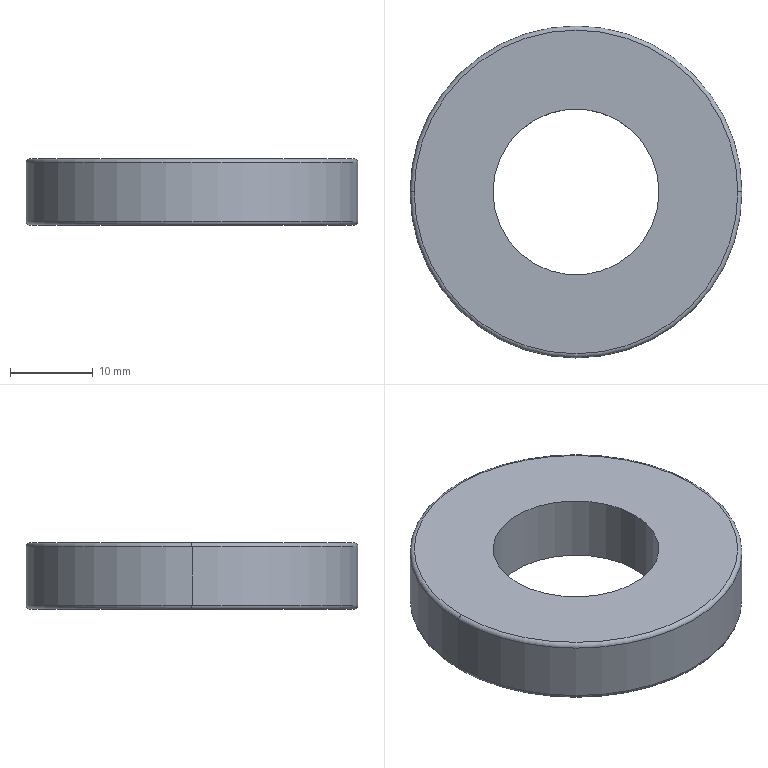Part | SolidWorks | features Extrusion 1, Fillet 1 | 1 solid | 10 faces | box 40 x 40 x 8 mm | volume 7526 mm3 | torus 4 | cylinder 4 | plane 2 | commonest cylinder face diameters 20 x2 40 x2
STEP:
#1=CARTESIAN_POINT('',(-20.,0.,3.5));
#2=VERTEX_POINT('',#1);
#3=CARTESIAN_POINT('',(20.,0.,3.5));
#4=VERTEX_POINT('',#3);
#5=CARTESIAN_POINT('',(0.,0.,3.5));
#6=DIRECTION('',(0.,0.,-1.));
#7=DIRECTION('',(1.,0.,0.));
#8=AXIS2_PLACEMENT_3D('',#5,#6,#7);
#9=CIRCLE('',#8,20.);
#10=EDGE_CURVE('',#2,#4,#9,.T.);
#11=ORIENTED_EDGE('',*,*,#10,.F.);
#12=CARTESIAN_POINT('',(-19.5,0.,4.));
#13=VERTEX_POINT('',#12);
#14=CARTESIAN_POINT('',(-19.5,0.,3.5));
#15=DIRECTION('',(0.,1.,0.));
#16=DIRECTION('',(-1.,0.,0.));
#17=AXIS2_PLACEMENT_3D('',#14,#15,#16);
#18=CIRCLE('',#17,0.5);
#19=EDGE_CURVE('',#2,#13,#18,.T.);
#20=ORIENTED_EDGE('',*,*,#19,.T.);
#21=CARTESIAN_POINT('',(19.5,0.,4.));
#22=VERTEX_POINT('',#21);
#23=CARTESIAN_POINT('',(0.,0.,4.));
#24=DIRECTION('',(0.,0.,1.));
#25=DIRECTION('',(1.,0.,0.));
#26=AXIS2_PLACEMENT_3D('',#23,#24,#25);
#27=CIRCLE('',#26,19.5);
#28=EDGE_CURVE('',#22,#13,#27,.T.);
#29=ORIENTED_EDGE('',*,*,#28,.F.);
#30=CARTESIAN_POINT('',(19.5,0.,3.5));
#31=DIRECTION('',(0.,-1.,0.));
#32=DIRECTION('',(0.,0.,-1.));
#33=AXIS2_PLACEMENT_3D('',#30,#31,#32);
#34=CIRCLE('',#33,0.5);
#35=EDGE_CURVE('',#4,#22,#34,.T.);
#36=ORIENTED_EDGE('',*,*,#35,.F.);
#37=EDGE_LOOP('',(#11,#20,#29,#36));
#38=FACE_OUTER_BOUND('',#37,.T.);
#39=CARTESIAN_POINT('',(0.,0.,3.5));
#40=DIRECTION('',(0.,0.,1.));
#41=DIRECTION('',(1.,0.,0.));
#42=AXIS2_PLACEMENT_3D('',#39,#40,#41);
#43=TOROIDAL_SURFACE('',#42,19.5,0.5);
#44=ADVANCED_FACE('',(#38),#43,.T.);
#45=CARTESIAN_POINT('',(-19.5,0.,-4.));
#46=VERTEX_POINT('',#45);
#47=CARTESIAN_POINT('',(19.5,0.,-4.));
#48=VERTEX_POINT('',#47);
#49=CARTESIAN_POINT('',(0.,0.,-4.));
#50=DIRECTION('',(0.,0.,-1.));
#51=DIRECTION('',(1.,0.,0.));
#52=AXIS2_PLACEMENT_3D('',#49,#50,#51);
#53=CIRCLE('',#52,19.5);
#54=EDGE_CURVE('',#46,#48,#53,.T.);
#55=ORIENTED_EDGE('',*,*,#54,.F.);
#56=CARTESIAN_POINT('',(-20.,0.,-3.5));
#57=VERTEX_POINT('',#56);
#58=CARTESIAN_POINT('',(-19.5,0.,-3.5));
#59=DIRECTION('',(0.,1.,0.));
#60=DIRECTION('',(-1.,0.,0.));
#61=AXIS2_PLACEMENT_3D('',#58,#59,#60);
#62=CIRCLE('',#61,0.5);
#63=EDGE_CURVE('',#46,#57,#62,.T.);
#64=ORIENTED_EDGE('',*,*,#63,.T.);
#65=CARTESIAN_POINT('',(20.,0.,-3.5));
#66=VERTEX_POINT('',#65);
#67=CARTESIAN_POINT('',(0.,0.,-3.5));
#68=DIRECTION('',(0.,0.,1.));
#69=DIRECTION('',(1.,0.,0.));
#70=AXIS2_PLACEMENT_3D('',#67,#68,#69);
#71=CIRCLE('',#70,20.);
#72=EDGE_CURVE('',#66,#57,#71,.T.);
#73=ORIENTED_EDGE('',*,*,#72,.F.);
#74=CARTESIAN_POINT('',(19.5,0.,-3.5));
#75=DIRECTION('',(0.,-1.,0.));
#76=DIRECTION('',(0.,0.,-1.));
#77=AXIS2_PLACEMENT_3D('',#74,#75,#76);
#78=CIRCLE('',#77,0.5);
#79=EDGE_CURVE('',#48,#66,#78,.T.);
#80=ORIENTED_EDGE('',*,*,#79,.F.);
#81=EDGE_LOOP('',(#55,#64,#73,#80));
#82=FACE_OUTER_BOUND('',#81,.T.);
#83=CARTESIAN_POINT('',(0.,0.,-3.5));
#84=DIRECTION('',(0.,0.,1.));
#85=DIRECTION('',(1.,0.,0.));
#86=AXIS2_PLACEMENT_3D('',#83,#84,#85);
#87=TOROIDAL_SURFACE('',#86,19.5,0.5);
#88=ADVANCED_FACE('',(#82),#87,.T.);
#89=CARTESIAN_POINT('',(-10.,0.,4.));
#90=VERTEX_POINT('',#89);
#91=CARTESIAN_POINT('',(10.,0.,4.));
#92=VERTEX_POINT('',#91);
#93=CARTESIAN_POINT('',(0.,0.,4.));
#94=DIRECTION('',(0.,0.,1.));
#95=DIRECTION('',(1.,0.,0.));
#96=AXIS2_PLACEMENT_3D('',#93,#94,#95);
#97=CIRCLE('',#96,10.);
#98=EDGE_CURVE('',#90,#92,#97,.T.);
#99=ORIENTED_EDGE('',*,*,#98,.T.);
#100=CARTESIAN_POINT('',(10.,0.,-4.));
#101=VERTEX_POINT('',#100);
#102=CARTESIAN_POINT('',(10.,0.,4.));
#103=DIRECTION('',(0.,0.,-1.));
#104=VECTOR('',#103,1000.);
#105=LINE('',#102,#104);
#106=EDGE_CURVE('',#92,#101,#105,.T.);
#107=ORIENTED_EDGE('',*,*,#106,.T.);
#108=CARTESIAN_POINT('',(-10.,0.,-4.));
#109=VERTEX_POINT('',#108);
#110=CARTESIAN_POINT('',(0.,0.,-4.));
#111=DIRECTION('',(0.,0.,1.));
#112=DIRECTION('',(1.,0.,0.));
#113=AXIS2_PLACEMENT_3D('',#110,#111,#112);
#114=CIRCLE('',#113,10.);
#115=EDGE_CURVE('',#109,#101,#114,.T.);
#116=ORIENTED_EDGE('',*,*,#115,.F.);
#117=CARTESIAN_POINT('',(-10.,0.,4.));
#118=DIRECTION('',(0.,0.,-1.));
#119=VECTOR('',#118,1000.);
#120=LINE('',#117,#119);
#121=EDGE_CURVE('',#90,#109,#120,.T.);
#122=ORIENTED_EDGE('',*,*,#121,.F.);
#123=EDGE_LOOP('',(#99,#107,#116,#122));
#124=FACE_OUTER_BOUND('',#123,.T.);
#125=CARTESIAN_POINT('',(0.,0.,4.));
#126=DIRECTION('',(0.,0.,-1.));
#127=DIRECTION('',(-1.,0.,0.));
#128=AXIS2_PLACEMENT_3D('',#125,#126,#127);
#129=CYLINDRICAL_SURFACE('',#128,10.);
#130=ADVANCED_FACE('',(#124),#129,.F.);
#131=ORIENTED_EDGE('',*,*,#10,.T.);
#132=CARTESIAN_POINT('',(20.,0.,4.));
#133=DIRECTION('',(0.,0.,-1.));
#134=VECTOR('',#133,1000.);
#135=LINE('',#132,#134);
#136=EDGE_CURVE('',#4,#66,#135,.T.);
#137=ORIENTED_EDGE('',*,*,#136,.T.);
#138=ORIENTED_EDGE('',*,*,#72,.T.);
#139=CARTESIAN_POINT('',(-20.,0.,4.));
#140=DIRECTION('',(0.,0.,-1.));
#141=VECTOR('',#140,1000.);
#142=LINE('',#139,#141);
#143=EDGE_CURVE('',#2,#57,#142,.T.);
#144=ORIENTED_EDGE('',*,*,#143,.F.);
#145=EDGE_LOOP('',(#131,#137,#138,#144));
#146=FACE_OUTER_BOUND('',#145,.T.);
#147=CARTESIAN_POINT('',(0.,0.,4.));
#148=DIRECTION('',(0.,0.,-1.));
#149=DIRECTION('',(-1.,0.,0.));
#150=AXIS2_PLACEMENT_3D('',#147,#148,#149);
#151=CYLINDRICAL_SURFACE('',#150,20.);
#152=ADVANCED_FACE('',(#146),#151,.T.);
#153=ORIENTED_EDGE('',*,*,#28,.T.);
#154=CARTESIAN_POINT('',(0.,0.,4.));
#155=DIRECTION('',(0.,0.,1.));
#156=DIRECTION('',(1.,0.,0.));
#157=AXIS2_PLACEMENT_3D('',#154,#155,#156);
#158=CIRCLE('',#157,19.5);
#159=EDGE_CURVE('',#13,#22,#158,.T.);
#160=ORIENTED_EDGE('',*,*,#159,.T.);
#161=EDGE_LOOP('',(#153,#160));
#162=FACE_OUTER_BOUND('',#161,.T.);
#163=ORIENTED_EDGE('',*,*,#98,.F.);
#164=CARTESIAN_POINT('',(0.,0.,4.));
#165=DIRECTION('',(0.,0.,1.));
#166=DIRECTION('',(1.,0.,0.));
#167=AXIS2_PLACEMENT_3D('',#164,#165,#166);
#168=CIRCLE('',#167,10.);
#169=EDGE_CURVE('',#92,#90,#168,.T.);
#170=ORIENTED_EDGE('',*,*,#169,.F.);
#171=EDGE_LOOP('',(#163,#170));
#172=FACE_BOUND('',#171,.T.);
#173=CARTESIAN_POINT('',(0.,0.,4.));
#174=DIRECTION('',(0.,0.,1.));
#175=DIRECTION('',(1.,0.,0.));
#176=AXIS2_PLACEMENT_3D('',#173,#174,#175);
#177=PLANE('',#176);
#178=ADVANCED_FACE('',(#162,#172),#177,.T.);
#179=CARTESIAN_POINT('',(0.,0.,-4.));
#180=DIRECTION('',(0.,0.,-1.));
#181=DIRECTION('',(1.,0.,0.));
#182=AXIS2_PLACEMENT_3D('',#179,#180,#181);
#183=CIRCLE('',#182,19.5);
#184=EDGE_CURVE('',#48,#46,#183,.T.);
#185=ORIENTED_EDGE('',*,*,#184,.T.);
#186=ORIENTED_EDGE('',*,*,#54,.T.);
#187=EDGE_LOOP('',(#185,#186));
#188=FACE_OUTER_BOUND('',#187,.T.);
#189=ORIENTED_EDGE('',*,*,#115,.T.);
#190=CARTESIAN_POINT('',(0.,0.,-4.));
#191=DIRECTION('',(0.,0.,1.));
#192=DIRECTION('',(1.,0.,0.));
#193=AXIS2_PLACEMENT_3D('',#190,#191,#192);
#194=CIRCLE('',#193,10.);
#195=EDGE_CURVE('',#101,#109,#194,.T.);
#196=ORIENTED_EDGE('',*,*,#195,.T.);
#197=EDGE_LOOP('',(#189,#196));
#198=FACE_BOUND('',#197,.T.);
#199=CARTESIAN_POINT('',(0.,0.,-4.));
#200=DIRECTION('',(0.,0.,1.));
#201=DIRECTION('',(1.,0.,0.));
#202=AXIS2_PLACEMENT_3D('',#199,#200,#201);
#203=PLANE('',#202);
#204=ADVANCED_FACE('',(#188,#198),#203,.F.);
#205=ORIENTED_EDGE('',*,*,#136,.F.);
#206=CARTESIAN_POINT('',(0.,0.,3.5));
#207=DIRECTION('',(0.,0.,-1.));
#208=DIRECTION('',(1.,0.,0.));
#209=AXIS2_PLACEMENT_3D('',#206,#207,#208);
#210=CIRCLE('',#209,20.);
#211=EDGE_CURVE('',#4,#2,#210,.T.);
#212=ORIENTED_EDGE('',*,*,#211,.T.);
#213=ORIENTED_EDGE('',*,*,#143,.T.);
#214=CARTESIAN_POINT('',(0.,0.,-3.5));
#215=DIRECTION('',(0.,0.,1.));
#216=DIRECTION('',(1.,0.,0.));
#217=AXIS2_PLACEMENT_3D('',#214,#215,#216);
#218=CIRCLE('',#217,20.);
#219=EDGE_CURVE('',#57,#66,#218,.T.);
#220=ORIENTED_EDGE('',*,*,#219,.T.);
#221=EDGE_LOOP('',(#205,#212,#213,#220));
#222=FACE_OUTER_BOUND('',#221,.T.);
#223=CARTESIAN_POINT('',(0.,0.,4.));
#224=DIRECTION('',(0.,0.,-1.));
#225=DIRECTION('',(-1.,0.,0.));
#226=AXIS2_PLACEMENT_3D('',#223,#224,#225);
#227=CYLINDRICAL_SURFACE('',#226,20.);
#228=ADVANCED_FACE('',(#222),#227,.T.);
#229=ORIENTED_EDGE('',*,*,#106,.F.);
#230=ORIENTED_EDGE('',*,*,#169,.T.);
#231=ORIENTED_EDGE('',*,*,#121,.T.);
#232=ORIENTED_EDGE('',*,*,#195,.F.);
#233=EDGE_LOOP('',(#229,#230,#231,#232));
#234=FACE_OUTER_BOUND('',#233,.T.);
#235=CARTESIAN_POINT('',(0.,0.,4.));
#236=DIRECTION('',(0.,0.,-1.));
#237=DIRECTION('',(-1.,0.,0.));
#238=AXIS2_PLACEMENT_3D('',#235,#236,#237);
#239=CYLINDRICAL_SURFACE('',#238,10.);
#240=ADVANCED_FACE('',(#234),#239,.F.);
#241=ORIENTED_EDGE('',*,*,#63,.F.);
#242=ORIENTED_EDGE('',*,*,#184,.F.);
#243=ORIENTED_EDGE('',*,*,#79,.T.);
#244=ORIENTED_EDGE('',*,*,#219,.F.);
#245=EDGE_LOOP('',(#241,#242,#243,#244));
#246=FACE_OUTER_BOUND('',#245,.T.);
#247=CARTESIAN_POINT('',(0.,0.,-3.5));
#248=DIRECTION('',(0.,0.,1.));
#249=DIRECTION('',(1.,0.,0.));
#250=AXIS2_PLACEMENT_3D('',#247,#248,#249);
#251=TOROIDAL_SURFACE('',#250,19.5,0.5);
#252=ADVANCED_FACE('',(#246),#251,.T.);
#253=ORIENTED_EDGE('',*,*,#19,.F.);
#254=ORIENTED_EDGE('',*,*,#211,.F.);
#255=ORIENTED_EDGE('',*,*,#35,.T.);
#256=ORIENTED_EDGE('',*,*,#159,.F.);
#257=EDGE_LOOP('',(#253,#254,#255,#256));
#258=FACE_OUTER_BOUND('',#257,.T.);
#259=CARTESIAN_POINT('',(0.,0.,3.5));
#260=DIRECTION('',(0.,0.,1.));
#261=DIRECTION('',(1.,0.,0.));
#262=AXIS2_PLACEMENT_3D('',#259,#260,#261);
#263=TOROIDAL_SURFACE('',#262,19.5,0.5);
#264=ADVANCED_FACE('',(#258),#263,.T.);
#265=CLOSED_SHELL('',(#44,#88,#130,#152,#178,#204,#228,#240,#252,#264));
#266=MANIFOLD_SOLID_BREP('',#265);
#267=CARTESIAN_POINT('',(0.,0.,0.));
#268=DIRECTION('',(0.,0.,1.));
#269=DIRECTION('',(1.,0.,0.));
#270=AXIS2_PLACEMENT_3D('',#267,#268,#269);
#271=(LENGTH_UNIT()NAMED_UNIT(*)SI_UNIT(.MILLI.,.METRE.));
#272=UNCERTAINTY_MEASURE_WITH_UNIT(LENGTH_MEASURE(0.00001),#271,'','');
#273=(NAMED_UNIT(*)PLANE_ANGLE_UNIT()SI_UNIT($,.RADIAN.));
#274=(NAMED_UNIT(*)SI_UNIT($,.STERADIAN.)SOLID_ANGLE_UNIT());
#275=(GEOMETRIC_REPRESENTATION_CONTEXT(3)GLOBAL_UNCERTAINTY_ASSIGNED_CONTEXT((#272))GLOBAL_UNIT_ASSIGNED_CONTEXT((#271,#273,#274))REPRESENTATION_CONTEXT('',''));
#276=ADVANCED_BREP_SHAPE_REPRESENTATION('',(#266,#270),#275);